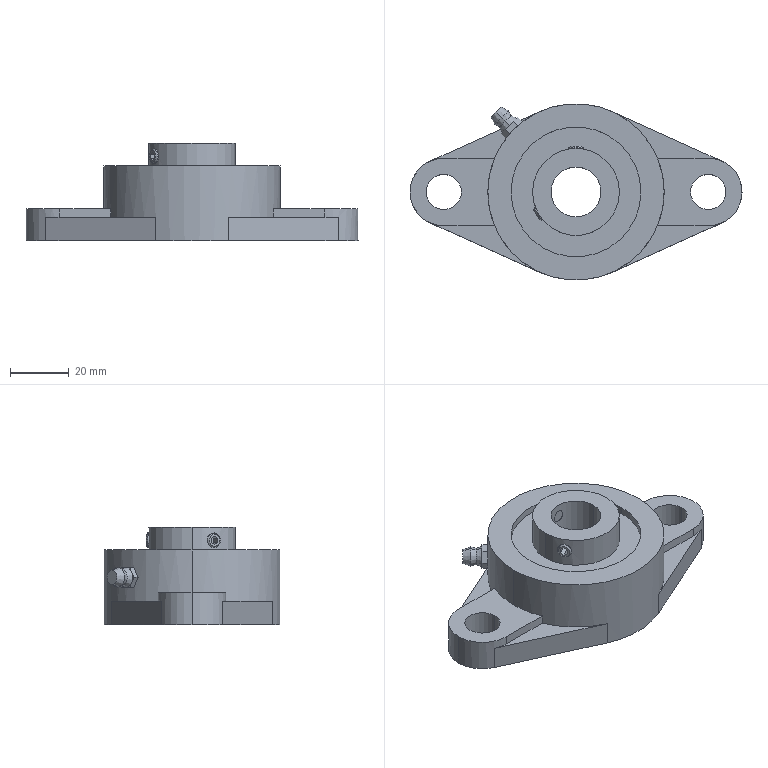Part | STEP file | UCFL203 | 2 solids | 100 faces | box 113 x 60 x 33.3 mm | volume 69003 mm3 | plane 58 | cylinder 32 | cone 10 | commonest cylinder face diameters 4.019 x5 23 x5 5 x4 12 x4 29.6 x4 60 x4